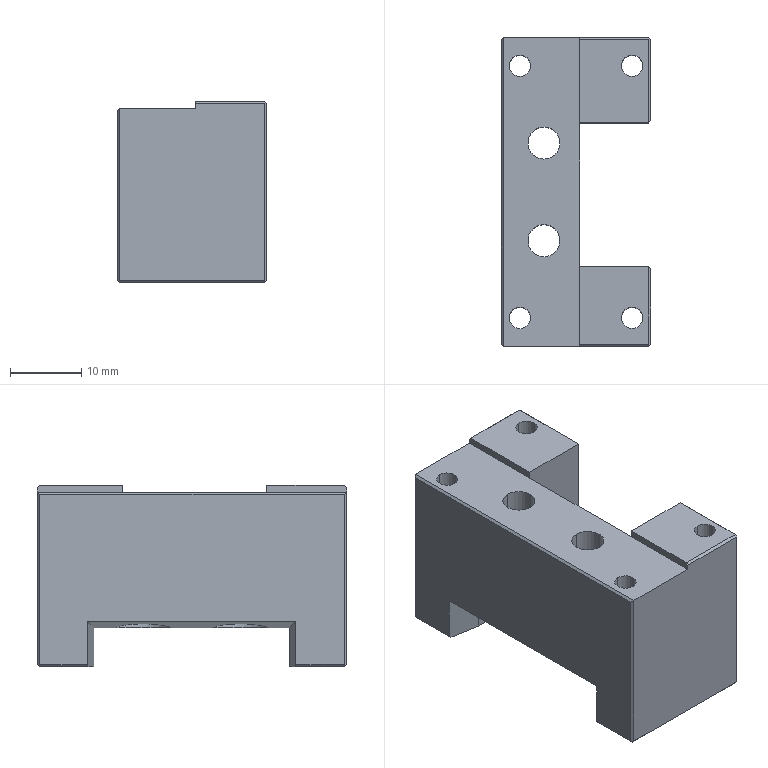Part | NX | 1 solid | 80 faces | box 21 x 43.4 x 25.5 mm | volume 13672 mm3 | plane 40 | cylinder 24 | cone 16 | commonest cylinder face diameters 2.5 x8 3 x8 4.5 x4 8 x4